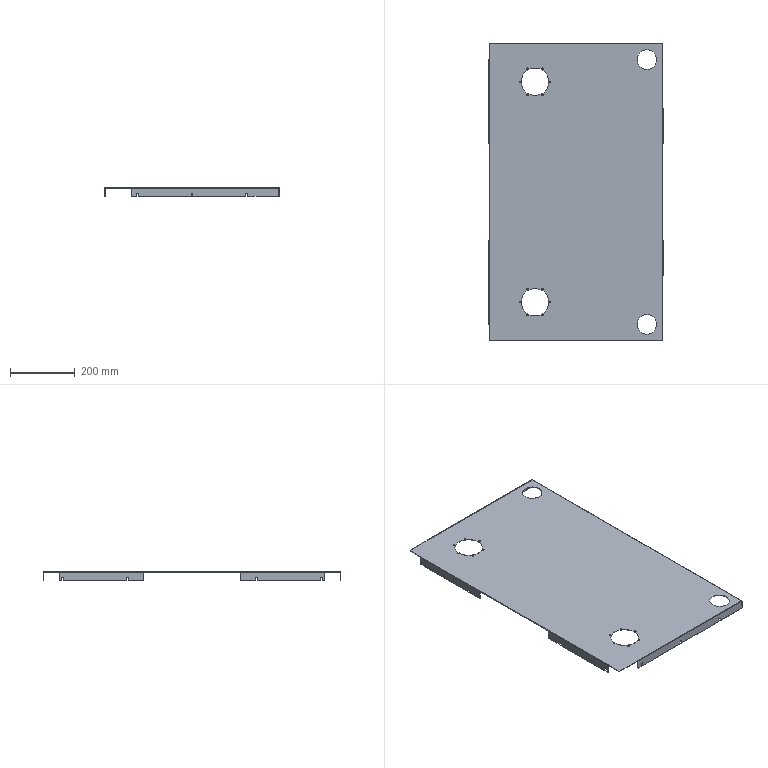Part | STEP file | upper cover plate 2 | 1 solid | 188 faces | box 537 x 917 x 27.5 mm | volume 772014 mm3 | cylinder 94 | plane 94 | commonest cylinder face diameters 2 x28 4.5 x24 6 x18 4 x8 0.02 x4 3.02 x4